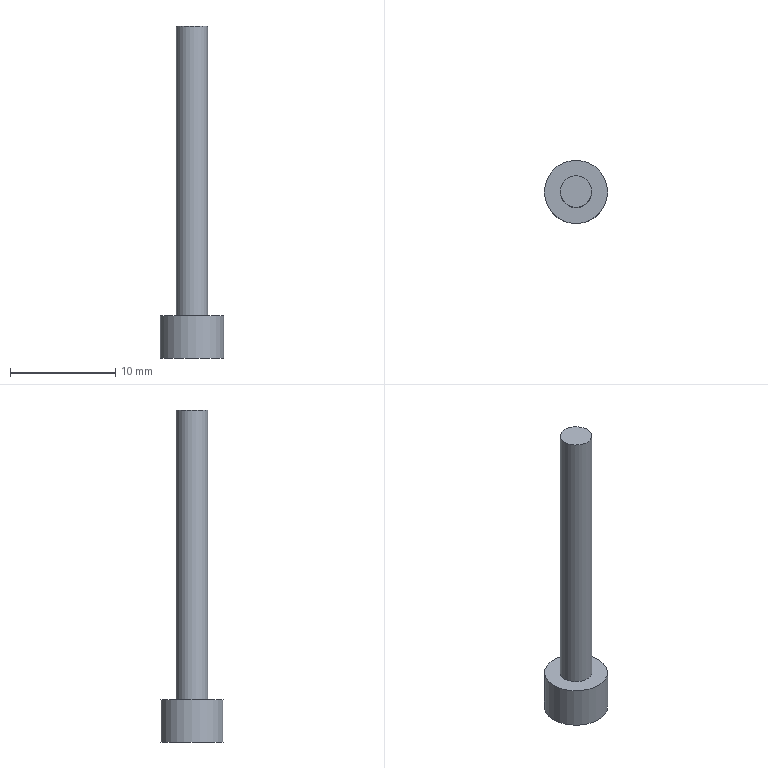Part | STEP file | 200 mesh_id1182 | 1 solid | 5 faces | box 6 x 6 x 31.5 mm | volume 307.483 mm3 | plane 3 | cylinder 2 | commonest cylinder face diameters 3 x1 6 x1
STEP:
#1=CARTESIAN_POINT('',(-16934.311,-4062.769,27.5));
#2=VERTEX_POINT('',#1);
#3=CARTESIAN_POINT('',(-16935.811,-4062.769,27.5));
#4=DIRECTION('',(0.,0.,-1.));
#5=DIRECTION('',(1.,0.,0.));
#6=AXIS2_PLACEMENT_3D('',#3,#4,#5);
#7=CIRCLE('',#6,1.5);
#8=EDGE_CURVE('',#2,#2,#7,.T.);
#9=ORIENTED_EDGE('',*,*,#8,.F.);
#10=EDGE_LOOP('',(#9));
#11=FACE_OUTER_BOUND('',#10,.T.);
#12=CARTESIAN_POINT('',(-16935.811,-4062.769,27.5));
#13=DIRECTION('',(0.,0.,1.));
#14=DIRECTION('',(1.,0.,0.));
#15=AXIS2_PLACEMENT_3D('',#12,#13,#14);
#16=PLANE('',#15);
#17=ADVANCED_FACE('',(#11),#16,.T.);
#18=ORIENTED_EDGE('',*,*,#8,.T.);
#19=EDGE_LOOP('',(#18));
#20=FACE_BOUND('',#19,.T.);
#21=CARTESIAN_POINT('',(-16934.311,-4062.769,0.));
#22=VERTEX_POINT('',#21);
#23=CARTESIAN_POINT('',(-16935.811,-4062.769,0.));
#24=DIRECTION('',(0.,0.,-1.));
#25=DIRECTION('',(1.,0.,0.));
#26=AXIS2_PLACEMENT_3D('',#23,#24,#25);
#27=CIRCLE('',#26,1.5);
#28=EDGE_CURVE('',#22,#22,#27,.T.);
#29=ORIENTED_EDGE('',*,*,#28,.F.);
#30=EDGE_LOOP('',(#29));
#31=FACE_BOUND('',#30,.T.);
#32=CARTESIAN_POINT('',(-16935.811,-4062.769,0.2));
#33=DIRECTION('',(0.,0.,1.));
#34=DIRECTION('',(1.,0.,0.));
#35=AXIS2_PLACEMENT_3D('',#32,#33,#34);
#36=CYLINDRICAL_SURFACE('',#35,1.5);
#37=ADVANCED_FACE('',(#20,#31),#36,.T.);
#38=CARTESIAN_POINT('',(-16938.811,-4062.769,-4.));
#39=VERTEX_POINT('',#38);
#40=CARTESIAN_POINT('',(-16935.811,-4062.769,-4.));
#41=DIRECTION('',(0.,0.,1.));
#42=DIRECTION('',(-1.,0.,0.));
#43=AXIS2_PLACEMENT_3D('',#40,#41,#42);
#44=CIRCLE('',#43,3.);
#45=EDGE_CURVE('',#39,#39,#44,.T.);
#46=ORIENTED_EDGE('',*,*,#45,.F.);
#47=EDGE_LOOP('',(#46));
#48=FACE_OUTER_BOUND('',#47,.T.);
#49=CARTESIAN_POINT('',(-16935.811,-4062.769,-4.));
#50=DIRECTION('',(0.,0.,-1.));
#51=DIRECTION('',(-1.,0.,0.));
#52=AXIS2_PLACEMENT_3D('',#49,#50,#51);
#53=PLANE('',#52);
#54=ADVANCED_FACE('',(#48),#53,.T.);
#55=ORIENTED_EDGE('',*,*,#28,.T.);
#56=EDGE_LOOP('',(#55));
#57=FACE_BOUND('',#56,.T.);
#58=CARTESIAN_POINT('',(-16932.811,-4062.769,0.));
#59=VERTEX_POINT('',#58);
#60=CARTESIAN_POINT('',(-16935.811,-4062.769,0.));
#61=DIRECTION('',(0.,0.,-1.));
#62=DIRECTION('',(1.,0.,0.));
#63=AXIS2_PLACEMENT_3D('',#60,#61,#62);
#64=CIRCLE('',#63,3.);
#65=EDGE_CURVE('',#59,#59,#64,.T.);
#66=ORIENTED_EDGE('',*,*,#65,.F.);
#67=EDGE_LOOP('',(#66));
#68=FACE_BOUND('',#67,.T.);
#69=CARTESIAN_POINT('',(-16935.811,-4062.769,0.));
#70=DIRECTION('',(0.,0.,1.));
#71=DIRECTION('',(1.,0.,0.));
#72=AXIS2_PLACEMENT_3D('',#69,#70,#71);
#73=PLANE('',#72);
#74=ADVANCED_FACE('',(#57,#68),#73,.T.);
#75=ORIENTED_EDGE('',*,*,#45,.T.);
#76=EDGE_LOOP('',(#75));
#77=FACE_BOUND('',#76,.T.);
#78=ORIENTED_EDGE('',*,*,#65,.T.);
#79=EDGE_LOOP('',(#78));
#80=FACE_BOUND('',#79,.T.);
#81=CARTESIAN_POINT('',(-16935.811,-4062.769,0.));
#82=DIRECTION('',(0.,0.,-1.));
#83=DIRECTION('',(1.,0.,0.));
#84=AXIS2_PLACEMENT_3D('',#81,#82,#83);
#85=CYLINDRICAL_SURFACE('',#84,3.);
#86=ADVANCED_FACE('',(#77,#80),#85,.T.);
#87=CLOSED_SHELL('',(#17,#37,#54,#74,#86));
#88=MANIFOLD_SOLID_BREP('',#87);
#89=(LENGTH_UNIT()NAMED_UNIT(*)SI_UNIT(.MILLI.,.METRE.));
#90=UNCERTAINTY_MEASURE_WITH_UNIT(LENGTH_MEASURE(0.00002),#89,'','');
#91=(NAMED_UNIT(*)PLANE_ANGLE_UNIT()SI_UNIT($,.RADIAN.));
#92=PLANE_ANGLE_MEASURE_WITH_UNIT(PLANE_ANGLE_MEASURE(0.01745),#91);
#93=DIMENSIONAL_EXPONENTS(0.,0.,0.,0.,0.,0.,0.);
#94=(CONVERSION_BASED_UNIT('DEGREE',#92)NAMED_UNIT(#93)PLANE_ANGLE_UNIT());
#95=(NAMED_UNIT(*)SI_UNIT($,.STERADIAN.)SOLID_ANGLE_UNIT());
#96=(GEOMETRIC_REPRESENTATION_CONTEXT(3)GLOBAL_UNCERTAINTY_ASSIGNED_CONTEXT((#90))GLOBAL_UNIT_ASSIGNED_CONTEXT((#89,#94,#95))REPRESENTATION_CONTEXT('',''));
#97=ADVANCED_BREP_SHAPE_REPRESENTATION('',(#88),#96);